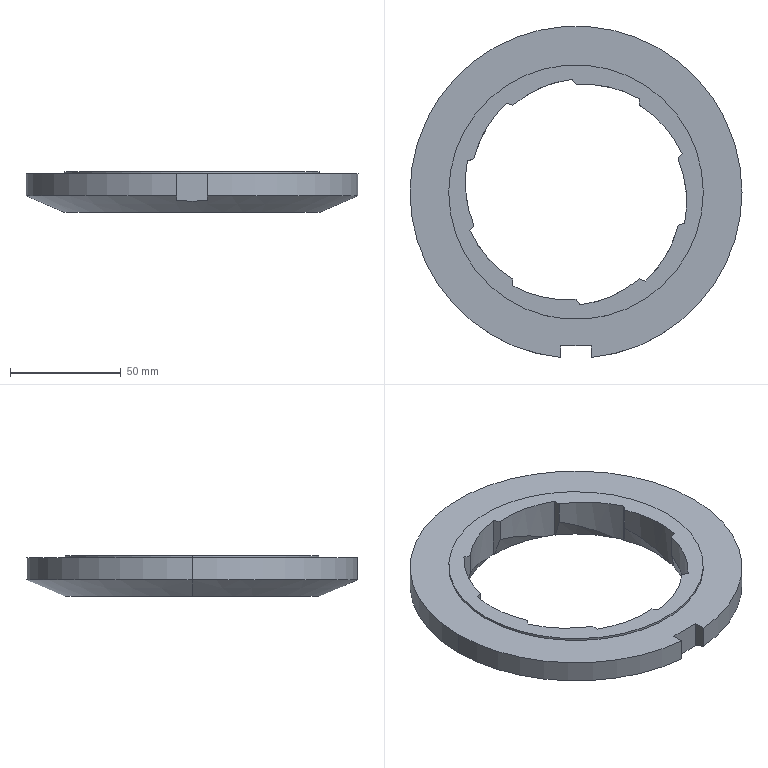Part | SolidWorks | features BaseBody 1, ICE 1 | 1 solid | 45 faces | box 150 x 149.673 x 18.5 mm | volume 145659 mm3 | cylinder 16 | plane 16 | cone 13 | commonest cylinder face diameters 100 x11 150 x3 115 x2